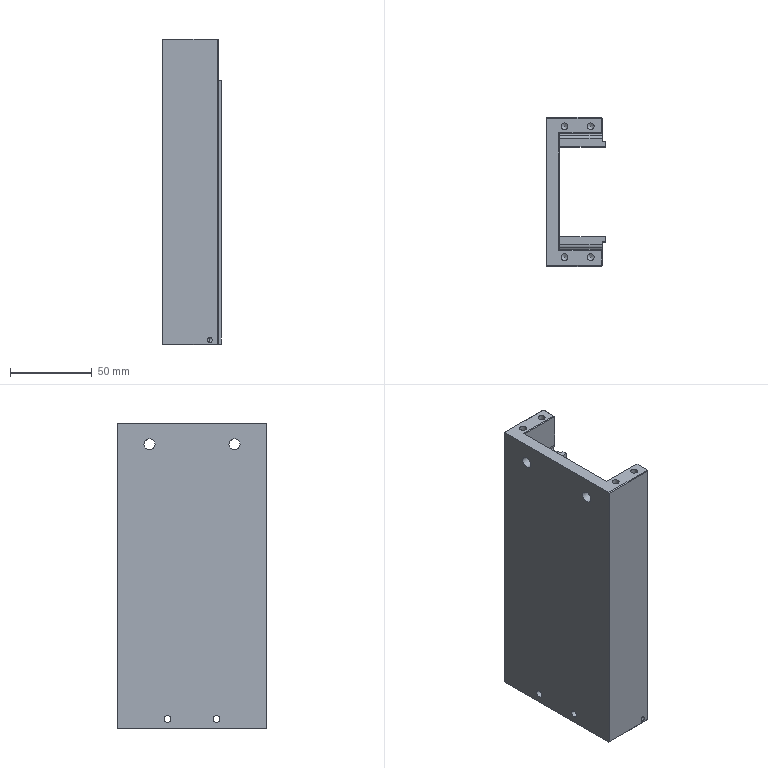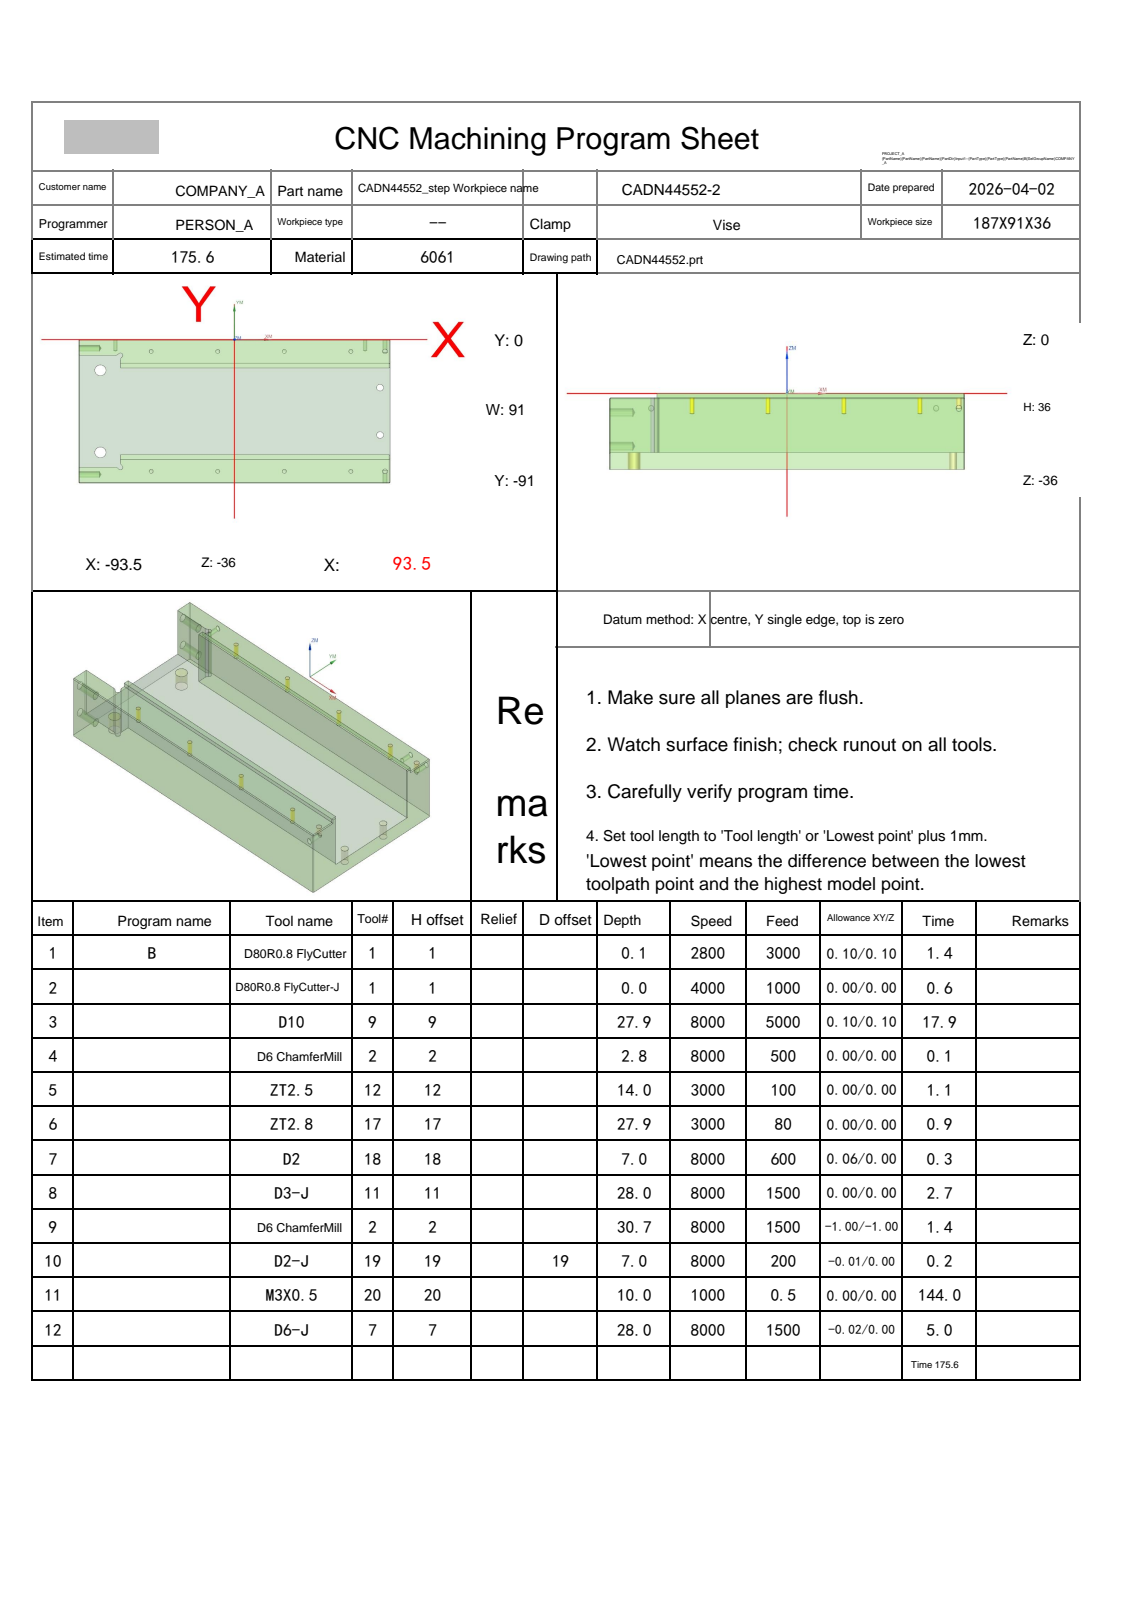NC program | NX | posted by the shop | part box 36 x 91 x 187 mm
Lines 5546 to 5692 of 12140:
N4 T02 M06
(D6 ChamferMill  D=6. R=0. H=02 ce=0.00 di=0.10)
G00 G90 G54 X90.5 Y-83.5 M03 S8000
G43 H02 Z20.
M08
G98 G81 X90.5 Y-83.5 Z-2.8 R-1. F500.
X70.
X30.
X-10.
X-50.
Y-7.5
X-10.
X30.
X70.
X90.5
X-68.5 Y-10.
Y-81.
G80
G00 Z20.
G91 G28 Z0.0
M05
M09
G91 G28 Z0.0
M01
N5 T12 M06
(ZT2.5 D=2.5 DR_a=118 H=12)
G00 G90 G54 X-50. Y-7.5 M03 S3000
G43 H12 Z20.
M08
G98 G83 X-50. Y-7.5 Z-14. R-1. F100. Q2.
X-10.
X30.
X70.
Y-83.5
X30.
X-10.
X-50.
G80
G00 Z20.
G91 G28 Z0.0
M05
M09
G91 G28 Z0.0
M01
N6 T17 M06
(ZT2.8 D=2.8 DR_a=118 H=17)
G00 G90 G54 X90.5 Y-7.5 M03 S3000
G43 H17 Z20.
M08
G98 G83 X90.5 Y-7.5 Z-6.9 R-1. F80. Q2.
G98 G83 X90.5 Y-83.5 Z-8.841 R-1. Q2.
G98 G83 X-68.5 Y-10. Z-27.9 R-1. Q2.
Y-81.
G80
G00 Z20.
G91 G28 Z0.0
M05
M09
G91 G28 Z0.0
M01
N7 T18 M06
(D2  D=2. R=0. H=18 ce=0.06 di=0.00)
G00 G90 G54 X90.5 Y-7.5 M03 S8000
G43 H18 Z20.
M08
Z-1.5
G03 X90.72 Y-7.28 I0.0 J.22 F600.
X90.5 Y-7.06 I-.22 J0.0
X90.5 Y-7.06 Z-1.7 I0.0 J-.44
X90.5 Y-7.06 Z-1.9 I0.0 J-.44
X90.5 Y-7.06 Z-2.1 I0.0 J-.44
X90.5 Y-7.06 Z-2.3 I0.0 J-.44
X90.5 Y-7.06 Z-2.5 I0.0 J-.44
X90.5 Y-7.06 Z-2.7 I0.0 J-.44
X90.5 Y-7.06 Z-2.9 I0.0 J-.44
X90.5 Y-7.06 Z-3.1 I0.0 J-.44
X90.5 Y-7.06 Z-3.3 I0.0 J-.44
X90.5 Y-7.06 Z-3.5 I0.0 J-.44
X90.5 Y-7.06 Z-3.7 I0.0 J-.44
X90.5 Y-7.06 Z-3.9 I0.0 J-.44
X90.5 Y-7.06 Z-4.1 I0.0 J-.44
X90.5 Y-7.06 Z-4.3 I0.0 J-.44
X90.5 Y-7.06 Z-4.5 I0.0 J-.44
X90.5 Y-7.06 Z-4.7 I0.0 J-.44
X90.5 Y-7.06 Z-4.9 I0.0 J-.44
X90.5 Y-7.06 Z-5.1 I0.0 J-.44
X90.5 Y-7.06 Z-5.3 I0.0 J-.44
X90.5 Y-7.06 Z-5.5 I0.0 J-.44
X90.5 Y-7.06 Z-5.7 I0.0 J-.44
X90.5 Y-7.06 Z-5.9 I0.0 J-.44
X90.5 Y-7.06 Z-6.1 I0.0 J-.44
X90.5 Y-7.06 Z-6.3 I0.0 J-.44
X90.5 Y-7.06 Z-6.5 I0.0 J-.44
X90.5 Y-7.06 Z-6.7 I0.0 J-.44
X90.5 Y-7.06 Z-6.9 I0.0 J-.44
X90.5 Y-7.94 Z-7. I0.0 J-.44
X90.94 Y-7.5 I0.0 J.44
X90.5 Y-7.06 I-.44 J0.0
X90.06 Y-7.5 I0.0 J-.44
X90.5 Y-7.94 I.44 J0.0
X90.72 Y-7.72 I0.0 J.22
X90.5 Y-7.5 I-.22 J0.0
G00 Z20.
Y-83.5
Z-1.5
G03 X90.72 Y-83.28 I0.0 J.22
X90.5 Y-83.06 I-.22 J0.0
X90.5 Y-83.06 Z-1.7 I0.0 J-.44
X90.5 Y-83.06 Z-1.9 I0.0 J-.44
X90.5 Y-83.06 Z-2.1 I0.0 J-.44
X90.5 Y-83.06 Z-2.3 I0.0 J-.44
X90.5 Y-83.06 Z-2.5 I0.0 J-.44
X90.5 Y-83.06 Z-2.7 I0.0 J-.44
X90.5 Y-83.06 Z-2.9 I0.0 J-.44
X90.5 Y-83.06 Z-3.1 I0.0 J-.44
X90.5 Y-83.06 Z-3.3 I0.0 J-.44
X90.5 Y-83.06 Z-3.5 I0.0 J-.44
X90.5 Y-83.06 Z-3.7 I0.0 J-.44
X90.5 Y-83.06 Z-3.9 I0.0 J-.44
X90.5 Y-83.06 Z-4.1 I0.0 J-.44
X90.5 Y-83.06 Z-4.3 I0.0 J-.44
X90.5 Y-83.06 Z-4.5 I0.0 J-.44
X90.5 Y-83.06 Z-4.7 I0.0 J-.44
X90.5 Y-83.06 Z-4.9 I0.0 J-.44
X90.5 Y-83.06 Z-5.1 I0.0 J-.44
X90.5 Y-83.06 Z-5.3 I0.0 J-.44
X90.5 Y-83.06 Z-5.5 I0.0 J-.44
X90.5 Y-83.06 Z-5.7 I0.0 J-.44
X90.5 Y-83.06 Z-5.9 I0.0 J-.44
X90.5 Y-83.06 Z-6.1 I0.0 J-.44
X90.5 Y-83.06 Z-6.3 I0.0 J-.44
X90.5 Y-83.06 Z-6.5 I0.0 J-.44
X90.5 Y-83.06 Z-6.7 I0.0 J-.44
X90.5 Y-83.06 Z-6.9 I0.0 J-.44
X90.5 Y-83.94 Z-7. I0.0 J-.44
X90.94 Y-83.5 I0.0 J.44
X90.5 Y-83.06 I-.44 J0.0
X90.06 Y-83.5 I0.0 J-.44
X90.5 Y-83.94 I.44 J0.0
X90.72 Y-83.72 I0.0 J.22
X90.5 Y-83.5 I-.22 J0.0
G00 Z20.
G91 G28 Z0.0
M05
M09
G91 G28 Z0.0
M01